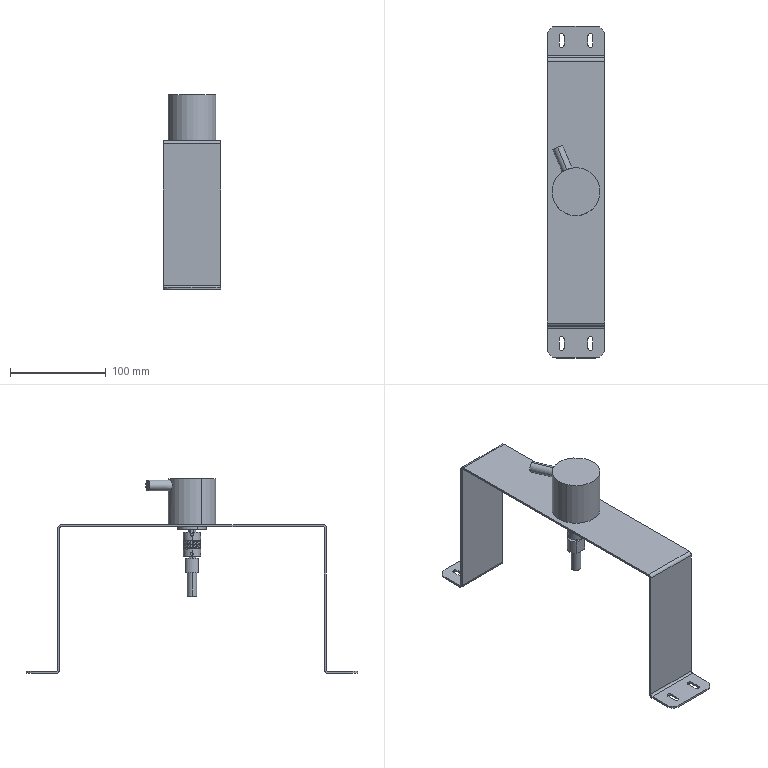Part | SolidWorks | 4 solids | 194 faces | box 60 x 346 x 203 mm | volume 185638 mm3 | cylinder 113 | plane 63 | cone 16 | spline 2 | commonest cylinder face diameters 8 x25 18 x19 4 x15 2.5 x12 3 x8 5 x8